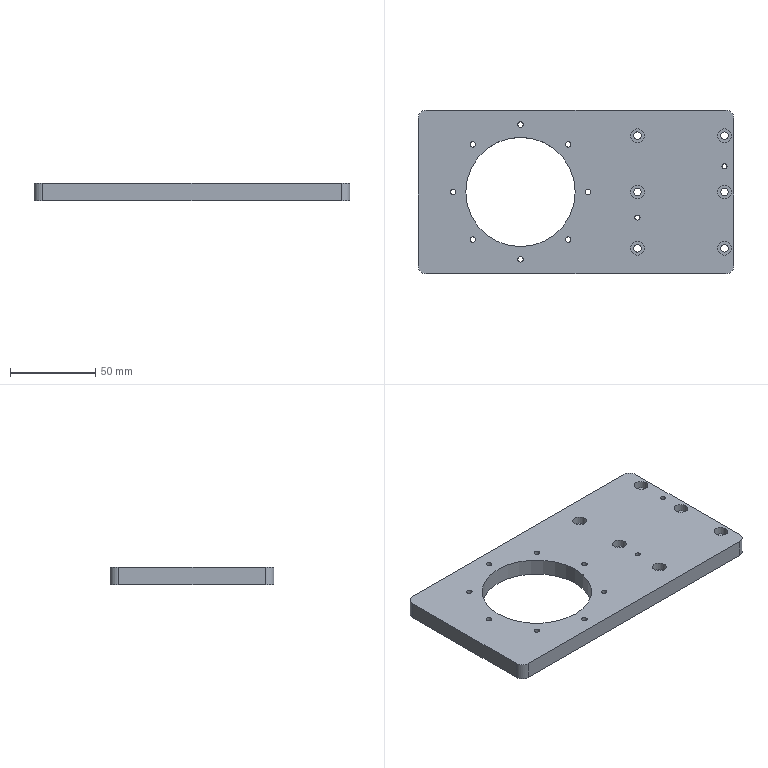Part | STEP file | SynoNew-0304-033 | 1 solid | 45 faces | box 185 x 96 x 10 mm | volume 142101 mm3 | cylinder 30 | plane 12 | cone 3 | commonest cylinder face diameters 3.242 x8 4.5 x6 8 x6 10 x4 4.2 x3 3 x2